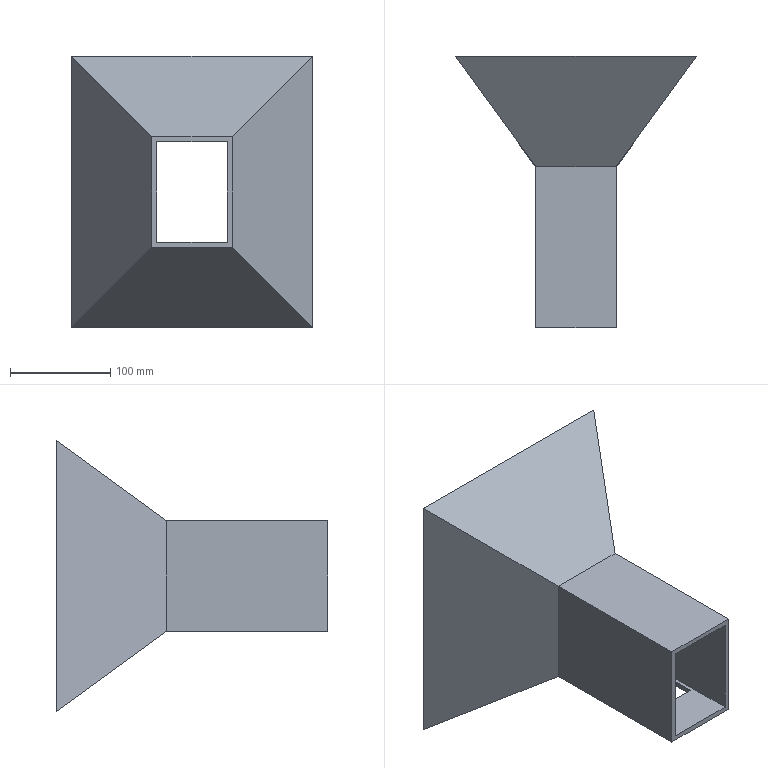Part | SolidWorks | features ICE 3, Blend 1, Extrusion 1, Shell 1 | 1 solid | 22 faces | box 240 x 270 x 270 mm | volume 740709 mm3 | plane 22
STEP:
#1=CARTESIAN_POINT('',(40.,0.,55.));
#2=VERTEX_POINT('',#1);
#3=CARTESIAN_POINT('',(40.,0.,-55.));
#4=VERTEX_POINT('',#3);
#5=CARTESIAN_POINT('',(40.,0.,-55.));
#6=DIRECTION('',(0.,0.,-1.));
#7=VECTOR('',#6,1000.);
#8=LINE('',#5,#7);
#9=EDGE_CURVE('',#2,#4,#8,.T.);
#10=ORIENTED_EDGE('',*,*,#9,.T.);
#11=CARTESIAN_POINT('',(40.,160.,-55.));
#12=VERTEX_POINT('',#11);
#13=CARTESIAN_POINT('',(40.,160.,-55.));
#14=DIRECTION('',(0.,-1.,0.));
#15=VECTOR('',#14,1000.);
#16=LINE('',#13,#15);
#17=EDGE_CURVE('',#12,#4,#16,.T.);
#18=ORIENTED_EDGE('',*,*,#17,.F.);
#19=CARTESIAN_POINT('',(40.,160.,55.));
#20=VERTEX_POINT('',#19);
#21=CARTESIAN_POINT('',(40.,160.,0.));
#22=DIRECTION('',(0.,0.,-1.));
#23=VECTOR('',#22,1000.);
#24=LINE('',#21,#23);
#25=EDGE_CURVE('',#20,#12,#24,.T.);
#26=ORIENTED_EDGE('',*,*,#25,.F.);
#27=CARTESIAN_POINT('',(40.,160.,55.));
#28=DIRECTION('',(0.,-1.,0.));
#29=VECTOR('',#28,1000.);
#30=LINE('',#27,#29);
#31=EDGE_CURVE('',#20,#2,#30,.T.);
#32=ORIENTED_EDGE('',*,*,#31,.T.);
#33=EDGE_LOOP('',(#10,#18,#26,#32));
#34=FACE_OUTER_BOUND('',#33,.T.);
#35=CARTESIAN_POINT('',(40.,160.,-55.));
#36=DIRECTION('',(-1.,0.,0.));
#37=DIRECTION('',(0.,0.,1.));
#38=AXIS2_PLACEMENT_3D('',#35,#36,#37);
#39=PLANE('',#38);
#40=ADVANCED_FACE('',(#34),#39,.F.);
#41=CARTESIAN_POINT('',(-31.,65.,-55.));
#42=VERTEX_POINT('',#41);
#43=CARTESIAN_POINT('',(31.,65.,-55.));
#44=VERTEX_POINT('',#43);
#45=CARTESIAN_POINT('',(31.,65.,-55.));
#46=DIRECTION('',(1.,0.,0.));
#47=VECTOR('',#46,1000.);
#48=LINE('',#45,#47);
#49=EDGE_CURVE('',#42,#44,#48,.T.);
#50=ORIENTED_EDGE('',*,*,#49,.F.);
#51=CARTESIAN_POINT('',(-31.,45.,-55.));
#52=VERTEX_POINT('',#51);
#53=CARTESIAN_POINT('',(-31.,45.,-55.));
#54=DIRECTION('',(0.,1.,0.));
#55=VECTOR('',#54,1000.);
#56=LINE('',#53,#55);
#57=EDGE_CURVE('',#52,#42,#56,.T.);
#58=ORIENTED_EDGE('',*,*,#57,.F.);
#59=CARTESIAN_POINT('',(31.,45.,-55.));
#60=VERTEX_POINT('',#59);
#61=CARTESIAN_POINT('',(31.,45.,-55.));
#62=DIRECTION('',(-1.,0.,0.));
#63=VECTOR('',#62,1000.);
#64=LINE('',#61,#63);
#65=EDGE_CURVE('',#60,#52,#64,.T.);
#66=ORIENTED_EDGE('',*,*,#65,.F.);
#67=CARTESIAN_POINT('',(31.,45.,-55.));
#68=DIRECTION('',(0.,-1.,0.));
#69=VECTOR('',#68,1000.);
#70=LINE('',#67,#69);
#71=EDGE_CURVE('',#44,#60,#70,.T.);
#72=ORIENTED_EDGE('',*,*,#71,.F.);
#73=EDGE_LOOP('',(#50,#58,#66,#72));
#74=FACE_BOUND('',#73,.T.);
#75=CARTESIAN_POINT('',(-40.,0.,-55.));
#76=VERTEX_POINT('',#75);
#77=CARTESIAN_POINT('',(-40.,0.,-55.));
#78=DIRECTION('',(-1.,0.,0.));
#79=VECTOR('',#78,1000.);
#80=LINE('',#77,#79);
#81=EDGE_CURVE('',#4,#76,#80,.T.);
#82=ORIENTED_EDGE('',*,*,#81,.T.);
#83=CARTESIAN_POINT('',(-40.,160.,-55.));
#84=VERTEX_POINT('',#83);
#85=CARTESIAN_POINT('',(-40.,160.,-55.));
#86=DIRECTION('',(0.,-1.,0.));
#87=VECTOR('',#86,1000.);
#88=LINE('',#85,#87);
#89=EDGE_CURVE('',#84,#76,#88,.T.);
#90=ORIENTED_EDGE('',*,*,#89,.F.);
#91=CARTESIAN_POINT('',(0.,160.,-55.));
#92=DIRECTION('',(-1.,0.,0.));
#93=VECTOR('',#92,1000.);
#94=LINE('',#91,#93);
#95=EDGE_CURVE('',#12,#84,#94,.T.);
#96=ORIENTED_EDGE('',*,*,#95,.F.);
#97=ORIENTED_EDGE('',*,*,#17,.T.);
#98=EDGE_LOOP('',(#82,#90,#96,#97));
#99=FACE_OUTER_BOUND('',#98,.T.);
#100=CARTESIAN_POINT('',(-40.,160.,-55.));
#101=DIRECTION('',(0.,0.,1.));
#102=DIRECTION('',(1.,0.,0.));
#103=AXIS2_PLACEMENT_3D('',#100,#101,#102);
#104=PLANE('',#103);
#105=ADVANCED_FACE('',(#74,#99),#104,.F.);
#106=CARTESIAN_POINT('',(-40.,0.,55.));
#107=VERTEX_POINT('',#106);
#108=CARTESIAN_POINT('',(-40.,0.,-55.));
#109=DIRECTION('',(0.,0.,1.));
#110=VECTOR('',#109,1000.);
#111=LINE('',#108,#110);
#112=EDGE_CURVE('',#76,#107,#111,.T.);
#113=ORIENTED_EDGE('',*,*,#112,.T.);
#114=CARTESIAN_POINT('',(-40.,160.,55.));
#115=VERTEX_POINT('',#114);
#116=CARTESIAN_POINT('',(-40.,160.,55.));
#117=DIRECTION('',(0.,-1.,0.));
#118=VECTOR('',#117,1000.);
#119=LINE('',#116,#118);
#120=EDGE_CURVE('',#115,#107,#119,.T.);
#121=ORIENTED_EDGE('',*,*,#120,.F.);
#122=CARTESIAN_POINT('',(-40.,160.,0.));
#123=DIRECTION('',(0.,0.,1.));
#124=VECTOR('',#123,1000.);
#125=LINE('',#122,#124);
#126=EDGE_CURVE('',#84,#115,#125,.T.);
#127=ORIENTED_EDGE('',*,*,#126,.F.);
#128=ORIENTED_EDGE('',*,*,#89,.T.);
#129=EDGE_LOOP('',(#113,#121,#127,#128));
#130=FACE_OUTER_BOUND('',#129,.T.);
#131=CARTESIAN_POINT('',(-40.,160.,-55.));
#132=DIRECTION('',(1.,0.,0.));
#133=DIRECTION('',(0.,0.,-1.));
#134=AXIS2_PLACEMENT_3D('',#131,#132,#133);
#135=PLANE('',#134);
#136=ADVANCED_FACE('',(#130),#135,.F.);
#137=CARTESIAN_POINT('',(-40.,0.,55.));
#138=DIRECTION('',(1.,0.,0.));
#139=VECTOR('',#138,1000.);
#140=LINE('',#137,#139);
#141=EDGE_CURVE('',#107,#2,#140,.T.);
#142=ORIENTED_EDGE('',*,*,#141,.T.);
#143=ORIENTED_EDGE('',*,*,#31,.F.);
#144=CARTESIAN_POINT('',(0.,160.,55.));
#145=DIRECTION('',(1.,0.,0.));
#146=VECTOR('',#145,1000.);
#147=LINE('',#144,#146);
#148=EDGE_CURVE('',#115,#20,#147,.T.);
#149=ORIENTED_EDGE('',*,*,#148,.F.);
#150=ORIENTED_EDGE('',*,*,#120,.T.);
#151=EDGE_LOOP('',(#142,#143,#149,#150));
#152=FACE_OUTER_BOUND('',#151,.T.);
#153=CARTESIAN_POINT('',(-40.,160.,55.));
#154=DIRECTION('',(0.,0.,-1.));
#155=DIRECTION('',(-1.,0.,0.));
#156=AXIS2_PLACEMENT_3D('',#153,#154,#155);
#157=PLANE('',#156);
#158=ADVANCED_FACE('',(#152),#157,.F.);
#159=CARTESIAN_POINT('',(-35.,0.,50.));
#160=VERTEX_POINT('',#159);
#161=CARTESIAN_POINT('',(35.,0.,50.));
#162=VERTEX_POINT('',#161);
#163=CARTESIAN_POINT('',(-40.,0.,50.));
#164=DIRECTION('',(1.,0.,0.));
#165=VECTOR('',#164,1000.);
#166=LINE('',#163,#165);
#167=EDGE_CURVE('',#160,#162,#166,.T.);
#168=ORIENTED_EDGE('',*,*,#167,.T.);
#169=CARTESIAN_POINT('',(35.,0.,-50.));
#170=VERTEX_POINT('',#169);
#171=CARTESIAN_POINT('',(35.,0.,-55.));
#172=DIRECTION('',(0.,0.,-1.));
#173=VECTOR('',#172,1000.);
#174=LINE('',#171,#173);
#175=EDGE_CURVE('',#162,#170,#174,.T.);
#176=ORIENTED_EDGE('',*,*,#175,.T.);
#177=CARTESIAN_POINT('',(-35.,0.,-50.));
#178=VERTEX_POINT('',#177);
#179=CARTESIAN_POINT('',(-40.,0.,-50.));
#180=DIRECTION('',(-1.,0.,0.));
#181=VECTOR('',#180,1000.);
#182=LINE('',#179,#181);
#183=EDGE_CURVE('',#170,#178,#182,.T.);
#184=ORIENTED_EDGE('',*,*,#183,.T.);
#185=CARTESIAN_POINT('',(-35.,0.,-55.));
#186=DIRECTION('',(0.,0.,1.));
#187=VECTOR('',#186,1000.);
#188=LINE('',#185,#187);
#189=EDGE_CURVE('',#178,#160,#188,.T.);
#190=ORIENTED_EDGE('',*,*,#189,.T.);
#191=EDGE_LOOP('',(#168,#176,#184,#190));
#192=FACE_BOUND('',#191,.T.);
#193=ORIENTED_EDGE('',*,*,#9,.F.);
#194=ORIENTED_EDGE('',*,*,#141,.F.);
#195=ORIENTED_EDGE('',*,*,#112,.F.);
#196=ORIENTED_EDGE('',*,*,#81,.F.);
#197=EDGE_LOOP('',(#193,#194,#195,#196));
#198=FACE_OUTER_BOUND('',#197,.T.);
#199=CARTESIAN_POINT('',(0.,0.,0.));
#200=DIRECTION('',(0.,1.,0.));
#201=DIRECTION('',(0.,0.,1.));
#202=AXIS2_PLACEMENT_3D('',#199,#200,#201);
#203=PLANE('',#202);
#204=ADVANCED_FACE('',(#192,#198),#203,.F.);
#205=CARTESIAN_POINT('',(-113.818,270.,-128.818));
#206=VERTEX_POINT('',#205);
#207=CARTESIAN_POINT('',(-113.818,270.,128.818));
#208=VERTEX_POINT('',#207);
#209=CARTESIAN_POINT('',(-113.818,270.,0.));
#210=DIRECTION('',(0.,0.,1.));
#211=VECTOR('',#210,1000.);
#212=LINE('',#209,#211);
#213=EDGE_CURVE('',#206,#208,#212,.T.);
#214=ORIENTED_EDGE('',*,*,#213,.F.);
#215=CARTESIAN_POINT('',(113.818,270.,-128.818));
#216=VERTEX_POINT('',#215);
#217=CARTESIAN_POINT('',(0.,270.,-128.818));
#218=DIRECTION('',(-1.,0.,0.));
#219=VECTOR('',#218,1000.);
#220=LINE('',#217,#219);
#221=EDGE_CURVE('',#216,#206,#220,.T.);
#222=ORIENTED_EDGE('',*,*,#221,.F.);
#223=CARTESIAN_POINT('',(113.818,270.,128.818));
#224=VERTEX_POINT('',#223);
#225=CARTESIAN_POINT('',(113.818,270.,0.));
#226=DIRECTION('',(0.,0.,-1.));
#227=VECTOR('',#226,1000.);
#228=LINE('',#225,#227);
#229=EDGE_CURVE('',#224,#216,#228,.T.);
#230=ORIENTED_EDGE('',*,*,#229,.F.);
#231=CARTESIAN_POINT('',(0.,270.,128.818));
#232=DIRECTION('',(1.,0.,0.));
#233=VECTOR('',#232,1000.);
#234=LINE('',#231,#233);
#235=EDGE_CURVE('',#208,#224,#234,.T.);
#236=ORIENTED_EDGE('',*,*,#235,.F.);
#237=EDGE_LOOP('',(#214,#222,#230,#236));
#238=FACE_BOUND('',#237,.T.);
#239=CARTESIAN_POINT('',(-120.,270.,-135.));
#240=VERTEX_POINT('',#239);
#241=CARTESIAN_POINT('',(-120.,270.,135.));
#242=VERTEX_POINT('',#241);
#243=CARTESIAN_POINT('',(-120.,270.,-135.));
#244=DIRECTION('',(0.,0.,1.));
#245=VECTOR('',#244,1000.);
#246=LINE('',#243,#245);
#247=EDGE_CURVE('',#240,#242,#246,.T.);
#248=ORIENTED_EDGE('',*,*,#247,.T.);
#249=CARTESIAN_POINT('',(120.,270.,135.));
#250=VERTEX_POINT('',#249);
#251=CARTESIAN_POINT('',(-120.,270.,135.));
#252=DIRECTION('',(1.,0.,0.));
#253=VECTOR('',#252,1000.);
#254=LINE('',#251,#253);
#255=EDGE_CURVE('',#242,#250,#254,.T.);
#256=ORIENTED_EDGE('',*,*,#255,.T.);
#257=CARTESIAN_POINT('',(120.,270.,-135.));
#258=VERTEX_POINT('',#257);
#259=CARTESIAN_POINT('',(120.,270.,135.));
#260=DIRECTION('',(0.,0.,-1.));
#261=VECTOR('',#260,1000.);
#262=LINE('',#259,#261);
#263=EDGE_CURVE('',#250,#258,#262,.T.);
#264=ORIENTED_EDGE('',*,*,#263,.T.);
#265=CARTESIAN_POINT('',(120.,270.,-135.));
#266=DIRECTION('',(-1.,0.,0.));
#267=VECTOR('',#266,1000.);
#268=LINE('',#265,#267);
#269=EDGE_CURVE('',#258,#240,#268,.T.);
#270=ORIENTED_EDGE('',*,*,#269,.T.);
#271=EDGE_LOOP('',(#248,#256,#264,#270));
#272=FACE_OUTER_BOUND('',#271,.T.);
#273=CARTESIAN_POINT('',(0.,270.,0.));
#274=DIRECTION('',(0.,1.,0.));
#275=DIRECTION('',(0.,0.,1.));
#276=AXIS2_PLACEMENT_3D('',#273,#274,#275);
#277=PLANE('',#276);
#278=ADVANCED_FACE('',(#238,#272),#277,.T.);
#279=CARTESIAN_POINT('',(-120.,270.,-135.));
#280=DIRECTION('',(0.507,-0.6971,0.507));
#281=VECTOR('',#280,1000.);
#282=LINE('',#279,#281);
#283=EDGE_CURVE('',#240,#84,#282,.T.);
#284=ORIENTED_EDGE('',*,*,#283,.T.);
#285=ORIENTED_EDGE('',*,*,#126,.T.);
#286=CARTESIAN_POINT('',(-120.,270.,135.));
#287=DIRECTION('',(0.507,-0.6971,-0.507));
#288=VECTOR('',#287,1000.);
#289=LINE('',#286,#288);
#290=EDGE_CURVE('',#242,#115,#289,.T.);
#291=ORIENTED_EDGE('',*,*,#290,.F.);
#292=ORIENTED_EDGE('',*,*,#247,.F.);
#293=EDGE_LOOP('',(#284,#285,#291,#292));
#294=FACE_OUTER_BOUND('',#293,.T.);
#295=CARTESIAN_POINT('',(49.946,36.324,0.));
#296=DIRECTION('',(0.8087,0.5882,0.));
#297=DIRECTION('',(-0.5882,0.8087,0.));
#298=AXIS2_PLACEMENT_3D('',#295,#296,#297);
#299=PLANE('',#298);
#300=ADVANCED_FACE('',(#294),#299,.F.);
#301=ORIENTED_EDGE('',*,*,#290,.T.);
#302=ORIENTED_EDGE('',*,*,#148,.T.);
#303=CARTESIAN_POINT('',(120.,270.,135.));
#304=DIRECTION('',(-0.507,-0.6971,-0.507));
#305=VECTOR('',#304,1000.);
#306=LINE('',#303,#305);
#307=EDGE_CURVE('',#250,#20,#306,.T.);
#308=ORIENTED_EDGE('',*,*,#307,.F.);
#309=ORIENTED_EDGE('',*,*,#255,.F.);
#310=EDGE_LOOP('',(#301,#302,#308,#309));
#311=FACE_OUTER_BOUND('',#310,.T.);
#312=CARTESIAN_POINT('',(0.,29.189,-40.135));
#313=DIRECTION('',(0.,0.5882,-0.8087));
#314=DIRECTION('',(0.,0.8087,0.5882));
#315=AXIS2_PLACEMENT_3D('',#312,#313,#314);
#316=PLANE('',#315);
#317=ADVANCED_FACE('',(#311),#316,.F.);
#318=CARTESIAN_POINT('',(120.,270.,-135.));
#319=DIRECTION('',(-0.507,-0.6971,0.507));
#320=VECTOR('',#319,1000.);
#321=LINE('',#318,#320);
#322=EDGE_CURVE('',#258,#12,#321,.T.);
#323=ORIENTED_EDGE('',*,*,#322,.T.);
#324=ORIENTED_EDGE('',*,*,#95,.T.);
#325=ORIENTED_EDGE('',*,*,#283,.F.);
#326=ORIENTED_EDGE('',*,*,#269,.F.);
#327=EDGE_LOOP('',(#323,#324,#325,#326));
#328=FACE_OUTER_BOUND('',#327,.T.);
#329=CARTESIAN_POINT('',(0.,29.189,40.135));
#330=DIRECTION('',(0.,0.5882,0.8087));
#331=DIRECTION('',(0.,-0.8087,0.5882));
#332=AXIS2_PLACEMENT_3D('',#329,#330,#331);
#333=PLANE('',#332);
#334=ADVANCED_FACE('',(#328),#333,.F.);
#335=ORIENTED_EDGE('',*,*,#307,.T.);
#336=ORIENTED_EDGE('',*,*,#25,.T.);
#337=ORIENTED_EDGE('',*,*,#322,.F.);
#338=ORIENTED_EDGE('',*,*,#263,.F.);
#339=EDGE_LOOP('',(#335,#336,#337,#338));
#340=FACE_OUTER_BOUND('',#339,.T.);
#341=CARTESIAN_POINT('',(-49.946,36.324,0.));
#342=DIRECTION('',(-0.8087,0.5882,0.));
#343=DIRECTION('',(-0.5882,-0.8087,0.));
#344=AXIS2_PLACEMENT_3D('',#341,#342,#343);
#345=PLANE('',#344);
#346=ADVANCED_FACE('',(#340),#345,.F.);
#347=ORIENTED_EDGE('',*,*,#175,.F.);
#348=CARTESIAN_POINT('',(35.,161.626,50.));
#349=VERTEX_POINT('',#348);
#350=CARTESIAN_POINT('',(35.,160.,50.));
#351=DIRECTION('',(0.,-1.,0.));
#352=VECTOR('',#351,1000.);
#353=LINE('',#350,#352);
#354=EDGE_CURVE('',#349,#162,#353,.T.);
#355=ORIENTED_EDGE('',*,*,#354,.F.);
#356=CARTESIAN_POINT('',(35.,161.626,-50.));
#357=VERTEX_POINT('',#356);
#358=CARTESIAN_POINT('',(35.,161.626,-55.));
#359=DIRECTION('',(0.,0.,-1.));
#360=VECTOR('',#359,1000.);
#361=LINE('',#358,#360);
#362=EDGE_CURVE('',#349,#357,#361,.T.);
#363=ORIENTED_EDGE('',*,*,#362,.T.);
#364=CARTESIAN_POINT('',(35.,160.,-50.));
#365=DIRECTION('',(0.,-1.,0.));
#366=VECTOR('',#365,1000.);
#367=LINE('',#364,#366);
#368=EDGE_CURVE('',#357,#170,#367,.T.);
#369=ORIENTED_EDGE('',*,*,#368,.T.);
#370=EDGE_LOOP('',(#347,#355,#363,#369));
#371=FACE_OUTER_BOUND('',#370,.T.);
#372=CARTESIAN_POINT('',(35.,160.,-55.));
#373=DIRECTION('',(-1.,0.,0.));
#374=DIRECTION('',(0.,0.,1.));
#375=AXIS2_PLACEMENT_3D('',#372,#373,#374);
#376=PLANE('',#375);
#377=ADVANCED_FACE('',(#371),#376,.T.);
#378=CARTESIAN_POINT('',(-31.,45.,-50.));
#379=VERTEX_POINT('',#378);
#380=CARTESIAN_POINT('',(-31.,65.,-50.));
#381=VERTEX_POINT('',#380);
#382=CARTESIAN_POINT('',(-31.,45.,-50.));
#383=DIRECTION('',(0.,1.,0.));
#384=VECTOR('',#383,1000.);
#385=LINE('',#382,#384);
#386=EDGE_CURVE('',#379,#381,#385,.T.);
#387=ORIENTED_EDGE('',*,*,#386,.T.);
#388=CARTESIAN_POINT('',(31.,65.,-50.));
#389=VERTEX_POINT('',#388);
#390=CARTESIAN_POINT('',(31.,65.,-50.));
#391=DIRECTION('',(1.,0.,0.));
#392=VECTOR('',#391,1000.);
#393=LINE('',#390,#392);
#394=EDGE_CURVE('',#381,#389,#393,.T.);
#395=ORIENTED_EDGE('',*,*,#394,.T.);
#396=CARTESIAN_POINT('',(31.,45.,-50.));
#397=VERTEX_POINT('',#396);
#398=CARTESIAN_POINT('',(31.,45.,-50.));
#399=DIRECTION('',(0.,-1.,0.));
#400=VECTOR('',#399,1000.);
#401=LINE('',#398,#400);
#402=EDGE_CURVE('',#389,#397,#401,.T.);
#403=ORIENTED_EDGE('',*,*,#402,.T.);
#404=CARTESIAN_POINT('',(31.,45.,-50.));
#405=DIRECTION('',(-1.,0.,0.));
#406=VECTOR('',#405,1000.);
#407=LINE('',#404,#406);
#408=EDGE_CURVE('',#397,#379,#407,.T.);
#409=ORIENTED_EDGE('',*,*,#408,.T.);
#410=EDGE_LOOP('',(#387,#395,#403,#409));
#411=FACE_BOUND('',#410,.T.);
#412=ORIENTED_EDGE('',*,*,#183,.F.);
#413=ORIENTED_EDGE('',*,*,#368,.F.);
#414=CARTESIAN_POINT('',(-35.,161.626,-50.));
#415=VERTEX_POINT('',#414);
#416=CARTESIAN_POINT('',(-40.,161.626,-50.));
#417=DIRECTION('',(-1.,0.,0.));
#418=VECTOR('',#417,1000.);
#419=LINE('',#416,#418);
#420=EDGE_CURVE('',#357,#415,#419,.T.);
#421=ORIENTED_EDGE('',*,*,#420,.T.);
#422=CARTESIAN_POINT('',(-35.,160.,-50.));
#423=DIRECTION('',(0.,-1.,0.));
#424=VECTOR('',#423,1000.);
#425=LINE('',#422,#424);
#426=EDGE_CURVE('',#415,#178,#425,.T.);
#427=ORIENTED_EDGE('',*,*,#426,.T.);
#428=EDGE_LOOP('',(#412,#413,#421,#427));
#429=FACE_OUTER_BOUND('',#428,.T.);
#430=CARTESIAN_POINT('',(-40.,160.,-50.));
#431=DIRECTION('',(0.,0.,1.));
#432=DIRECTION('',(1.,0.,0.));
#433=AXIS2_PLACEMENT_3D('',#430,#431,#432);
#434=PLANE('',#433);
#435=ADVANCED_FACE('',(#411,#429),#434,.T.);
#436=ORIENTED_EDGE('',*,*,#189,.F.);
#437=ORIENTED_EDGE('',*,*,#426,.F.);
#438=CARTESIAN_POINT('',(-35.,161.626,50.));
#439=VERTEX_POINT('',#438);
#440=CARTESIAN_POINT('',(-35.,161.626,-55.));
#441=DIRECTION('',(0.,0.,1.));
#442=VECTOR('',#441,1000.);
#443=LINE('',#440,#442);
#444=EDGE_CURVE('',#415,#439,#443,.T.);
#445=ORIENTED_EDGE('',*,*,#444,.T.);
#446=CARTESIAN_POINT('',(-35.,160.,50.));
#447=DIRECTION('',(0.,-1.,0.));
#448=VECTOR('',#447,1000.);
#449=LINE('',#446,#448);
#450=EDGE_CURVE('',#439,#160,#449,.T.);
#451=ORIENTED_EDGE('',*,*,#450,.T.);
#452=EDGE_LOOP('',(#436,#437,#445,#451));
#453=FACE_OUTER_BOUND('',#452,.T.);
#454=CARTESIAN_POINT('',(-35.,160.,-55.));
#455=DIRECTION('',(1.,0.,0.));
#456=DIRECTION('',(0.,0.,-1.));
#457=AXIS2_PLACEMENT_3D('',#454,#455,#456);
#458=PLANE('',#457);
#459=ADVANCED_FACE('',(#453),#458,.T.);
#460=ORIENTED_EDGE('',*,*,#167,.F.);
#461=ORIENTED_EDGE('',*,*,#450,.F.);
#462=CARTESIAN_POINT('',(-40.,161.626,50.));
#463=DIRECTION('',(1.,0.,0.));
#464=VECTOR('',#463,1000.);
#465=LINE('',#462,#464);
#466=EDGE_CURVE('',#439,#349,#465,.T.);
#467=ORIENTED_EDGE('',*,*,#466,.T.);
#468=ORIENTED_EDGE('',*,*,#354,.T.);
#469=EDGE_LOOP('',(#460,#461,#467,#468));
#470=FACE_OUTER_BOUND('',#469,.T.);
#471=CARTESIAN_POINT('',(-40.,160.,50.));
#472=DIRECTION('',(0.,0.,-1.));
#473=DIRECTION('',(-1.,0.,0.));
#474=AXIS2_PLACEMENT_3D('',#471,#472,#473);
#475=PLANE('',#474);
#476=ADVANCED_FACE('',(#470),#475,.T.);
#477=CARTESIAN_POINT('',(43.968,53.045,28.968));
#478=DIRECTION('',(0.507,-0.6971,0.507));
#479=VECTOR('',#478,1000.);
#480=LINE('',#477,#479);
#481=EDGE_CURVE('',#206,#415,#480,.T.);
#482=ORIENTED_EDGE('',*,*,#481,.F.);
#483=ORIENTED_EDGE('',*,*,#213,.T.);
#484=CARTESIAN_POINT('',(43.968,53.045,-28.968));
#485=DIRECTION('',(0.507,-0.6971,-0.507));
#486=VECTOR('',#485,1000.);
#487=LINE('',#484,#486);
#488=EDGE_CURVE('',#208,#439,#487,.T.);
#489=ORIENTED_EDGE('',*,*,#488,.T.);
#490=ORIENTED_EDGE('',*,*,#444,.F.);
#491=EDGE_LOOP('',(#482,#483,#489,#490));
#492=FACE_OUTER_BOUND('',#491,.T.);
#493=CARTESIAN_POINT('',(53.99,39.265,0.));
#494=DIRECTION('',(0.8087,0.5882,0.));
#495=DIRECTION('',(-0.5882,0.8087,0.));
#496=AXIS2_PLACEMENT_3D('',#493,#494,#495);
#497=PLANE('',#496);
#498=ADVANCED_FACE('',(#492),#497,.T.);
#499=ORIENTED_EDGE('',*,*,#488,.F.);
#500=ORIENTED_EDGE('',*,*,#235,.T.);
#501=CARTESIAN_POINT('',(-43.968,53.045,-28.968));
#502=DIRECTION('',(-0.507,-0.6971,-0.507));
#503=VECTOR('',#502,1000.);
#504=LINE('',#501,#503);
#505=EDGE_CURVE('',#224,#349,#504,.T.);
#506=ORIENTED_EDGE('',*,*,#505,.T.);
#507=ORIENTED_EDGE('',*,*,#466,.F.);
#508=EDGE_LOOP('',(#499,#500,#506,#507));
#509=FACE_OUTER_BOUND('',#508,.T.);
#510=CARTESIAN_POINT('',(0.,32.13,-44.179));
#511=DIRECTION('',(0.,0.5882,-0.8087));
#512=DIRECTION('',(0.,0.8087,0.5882));
#513=AXIS2_PLACEMENT_3D('',#510,#511,#512);
#514=PLANE('',#513);
#515=ADVANCED_FACE('',(#509),#514,.T.);
#516=CARTESIAN_POINT('',(-43.968,53.045,28.968));
#517=DIRECTION('',(-0.507,-0.6971,0.507));
#518=VECTOR('',#517,1000.);
#519=LINE('',#516,#518);
#520=EDGE_CURVE('',#216,#357,#519,.T.);
#521=ORIENTED_EDGE('',*,*,#520,.F.);
#522=ORIENTED_EDGE('',*,*,#221,.T.);
#523=ORIENTED_EDGE('',*,*,#481,.T.);
#524=ORIENTED_EDGE('',*,*,#420,.F.);
#525=EDGE_LOOP('',(#521,#522,#523,#524));
#526=FACE_OUTER_BOUND('',#525,.T.);
#527=CARTESIAN_POINT('',(0.,32.13,44.179));
#528=DIRECTION('',(0.,0.5882,0.8087));
#529=DIRECTION('',(0.,-0.8087,0.5882));
#530=AXIS2_PLACEMENT_3D('',#527,#528,#529);
#531=PLANE('',#530);
#532=ADVANCED_FACE('',(#526),#531,.T.);
#533=ORIENTED_EDGE('',*,*,#505,.F.);
#534=ORIENTED_EDGE('',*,*,#229,.T.);
#535=ORIENTED_EDGE('',*,*,#520,.T.);
#536=ORIENTED_EDGE('',*,*,#362,.F.);
#537=EDGE_LOOP('',(#533,#534,#535,#536));
#538=FACE_OUTER_BOUND('',#537,.T.);
#539=CARTESIAN_POINT('',(-53.99,39.265,0.));
#540=DIRECTION('',(-0.8087,0.5882,0.));
#541=DIRECTION('',(-0.5882,-0.8087,0.));
#542=AXIS2_PLACEMENT_3D('',#539,#540,#541);
#543=PLANE('',#542);
#544=ADVANCED_FACE('',(#538),#543,.T.);
#545=ORIENTED_EDGE('',*,*,#57,.T.);
#546=CARTESIAN_POINT('',(-31.,65.,-50.));
#547=DIRECTION('',(0.,0.,-1.));
#548=VECTOR('',#547,1000.);
#549=LINE('',#546,#548);
#550=EDGE_CURVE('',#381,#42,#549,.T.);
#551=ORIENTED_EDGE('',*,*,#550,.F.);
#552=ORIENTED_EDGE('',*,*,#386,.F.);
#553=CARTESIAN_POINT('',(-31.,45.,-50.));
#554=DIRECTION('',(0.,0.,-1.));
#555=VECTOR('',#554,1000.);
#556=LINE('',#553,#555);
#557=EDGE_CURVE('',#379,#52,#556,.T.);
#558=ORIENTED_EDGE('',*,*,#557,.T.);
#559=EDGE_LOOP('',(#545,#551,#552,#558));
#560=FACE_OUTER_BOUND('',#559,.T.);
#561=CARTESIAN_POINT('',(-31.,45.,-50.));
#562=DIRECTION('',(-1.,0.,0.));
#563=DIRECTION('',(0.,-1.,0.));
#564=AXIS2_PLACEMENT_3D('',#561,#562,#563);
#565=PLANE('',#564);
#566=ADVANCED_FACE('',(#560),#565,.F.);
#567=ORIENTED_EDGE('',*,*,#65,.T.);
#568=ORIENTED_EDGE('',*,*,#557,.F.);
#569=ORIENTED_EDGE('',*,*,#408,.F.);
#570=CARTESIAN_POINT('',(31.,45.,-50.));
#571=DIRECTION('',(0.,0.,-1.));
#572=VECTOR('',#571,1000.);
#573=LINE('',#570,#572);
#574=EDGE_CURVE('',#397,#60,#573,.T.);
#575=ORIENTED_EDGE('',*,*,#574,.T.);
#576=EDGE_LOOP('',(#567,#568,#569,#575));
#577=FACE_OUTER_BOUND('',#576,.T.);
#578=CARTESIAN_POINT('',(31.,45.,-50.));
#579=DIRECTION('',(0.,-1.,0.));
#580=DIRECTION('',(0.,0.,-1.));
#581=AXIS2_PLACEMENT_3D('',#578,#579,#580);
#582=PLANE('',#581);
#583=ADVANCED_FACE('',(#577),#582,.F.);
#584=ORIENTED_EDGE('',*,*,#71,.T.);
#585=ORIENTED_EDGE('',*,*,#574,.F.);
#586=ORIENTED_EDGE('',*,*,#402,.F.);
#587=CARTESIAN_POINT('',(31.,65.,-50.));
#588=DIRECTION('',(0.,0.,-1.));
#589=VECTOR('',#588,1000.);
#590=LINE('',#587,#589);
#591=EDGE_CURVE('',#389,#44,#590,.T.);
#592=ORIENTED_EDGE('',*,*,#591,.T.);
#593=EDGE_LOOP('',(#584,#585,#586,#592));
#594=FACE_OUTER_BOUND('',#593,.T.);
#595=CARTESIAN_POINT('',(31.,45.,-50.));
#596=DIRECTION('',(1.,0.,0.));
#597=DIRECTION('',(0.,1.,0.));
#598=AXIS2_PLACEMENT_3D('',#595,#596,#597);
#599=PLANE('',#598);
#600=ADVANCED_FACE('',(#594),#599,.F.);
#601=ORIENTED_EDGE('',*,*,#49,.T.);
#602=ORIENTED_EDGE('',*,*,#591,.F.);
#603=ORIENTED_EDGE('',*,*,#394,.F.);
#604=ORIENTED_EDGE('',*,*,#550,.T.);
#605=EDGE_LOOP('',(#601,#602,#603,#604));
#606=FACE_OUTER_BOUND('',#605,.T.);
#607=CARTESIAN_POINT('',(31.,65.,-50.));
#608=DIRECTION('',(0.,1.,0.));
#609=DIRECTION('',(0.,0.,1.));
#610=AXIS2_PLACEMENT_3D('',#607,#608,#609);
#611=PLANE('',#610);
#612=ADVANCED_FACE('',(#606),#611,.F.);
#613=CLOSED_SHELL('',(#40,#105,#136,#158,#204,#278,#300,#317,#334,#346,#377,#435,#459,#476,#498,#515,#532,#544,#566,#583,#600,#612));
#614=MANIFOLD_SOLID_BREP('',#613);
#615=CARTESIAN_POINT('',(0.,0.,0.));
#616=DIRECTION('',(0.,0.,1.));
#617=DIRECTION('',(1.,0.,0.));
#618=AXIS2_PLACEMENT_3D('',#615,#616,#617);
#619=(LENGTH_UNIT()NAMED_UNIT(*)SI_UNIT(.MILLI.,.METRE.));
#620=UNCERTAINTY_MEASURE_WITH_UNIT(LENGTH_MEASURE(0.00001),#619,'','');
#621=(NAMED_UNIT(*)PLANE_ANGLE_UNIT()SI_UNIT($,.RADIAN.));
#622=(NAMED_UNIT(*)SI_UNIT($,.STERADIAN.)SOLID_ANGLE_UNIT());
#623=(GEOMETRIC_REPRESENTATION_CONTEXT(3)GLOBAL_UNCERTAINTY_ASSIGNED_CONTEXT((#620))GLOBAL_UNIT_ASSIGNED_CONTEXT((#619,#621,#622))REPRESENTATION_CONTEXT('',''));
#624=ADVANCED_BREP_SHAPE_REPRESENTATION('',(#614,#618),#623);